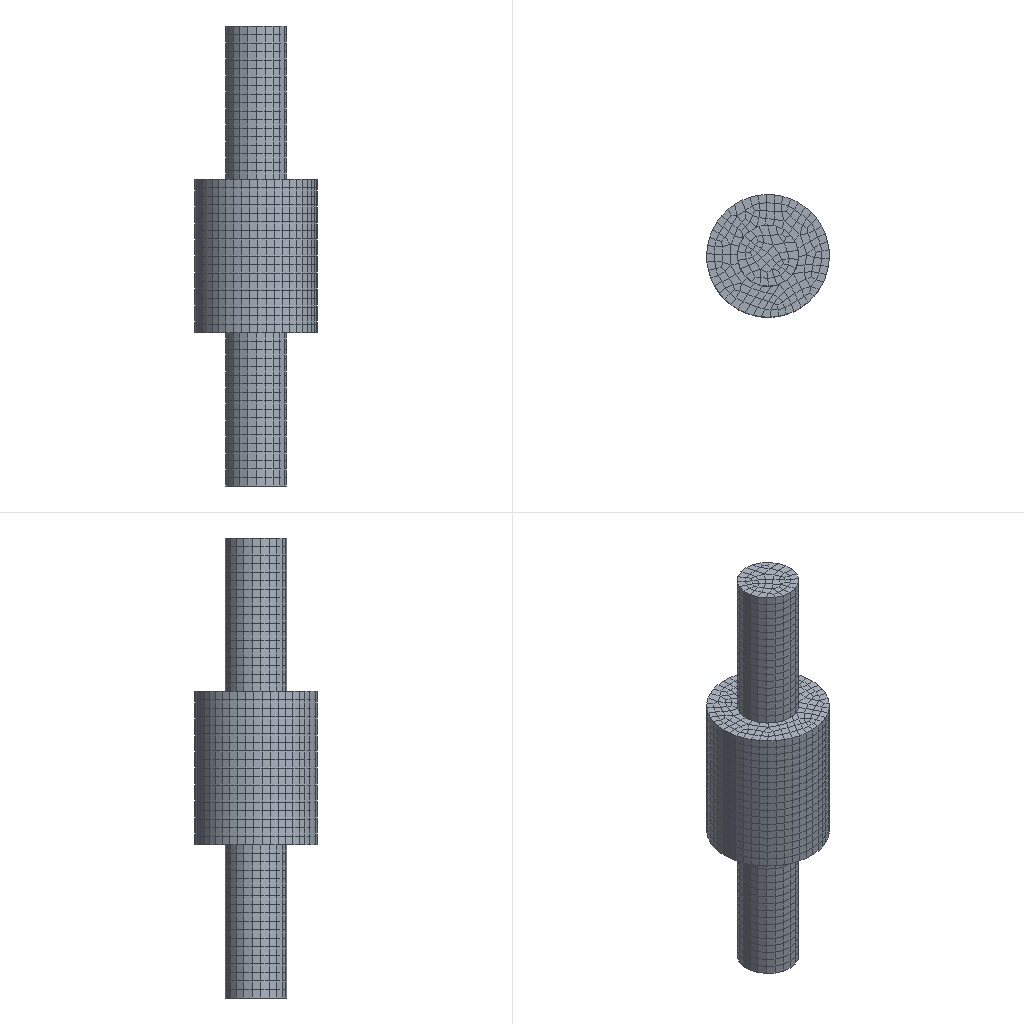Simulation study | abaqus
Set-up summary:
category,name,step,type,value,unit,region
solver,abaqus
solver,version,,,Abaqus/Standard 2020
units,not stated in the deck,,not stated
analysis,deck,,transient,transient
load_step,Step-1,Step-1,transient
load_step,requested,,,1
mesh,nodes,,,7238
mesh,elements,,,5724
element_type,C3D8R,,solid,5724
load,load commands in deck,,count,2
bc,support commands in deck,,count,6
material,MATERIAL-1,,in results
check,setup vs results,,match,"per instance, exact: element labels, types and connectivity; labels of the nodes the elements use; coordinates of those nodes at SINGLE_PRECISION in 2 of 2 instance(s)"
Abaqus input file, long lists of numbers shortened:
*Heading
** Job name: Job-1 Model name: Model-1
** Generated by: Abaqus/CAE 2020
*Preprint, echo=NO, model=NO, history=NO, contact=NO
**
** PARTS
**
*Part, name=Part-1
*Node
      1,   9.165,  -4.001,           0.
      2,   9.921,  -1.257,           0.
** (3683 more lines like these left out)
*Element, type=C3D8R
   1,  107,   89,   79,   91,   40,   22,   12,   24
   2,  106,   78,   88,   92,   39,   11,   21,   25
** (2968 more lines like these left out)
*Nset, nset=Set-1, generate
    1,  3685,     1
*Elset, elset=Set-1, generate
    1,  2970,     1
** Section: Section-1
*Solid Section, elset=Set-1, material=Material-1
,
*End Part
**
*Part, name=tong
*Node
      1,   8.194,  -5.732,           0.
      2,   9.477,  -3.192,           0.
** (3551 more lines like these left out)
*Element, type=C3D8R
   1,  301,  233,  191,  259,  114,   46,    4,   72
   2,  356,  308,  257,  337,  169,  121,   70,  150
** (2752 more lines like these left out)
*Nset, nset=Set-1, generate
    1,  3553,     1
*Elset, elset=Set-1, generate
    1,  2754,     1
** Section: Section-1
*Solid Section, elset=Set-1, material=Material-1
,
*End Part
**
**
** ASSEMBLY
**
*Assembly, name=Assembly
**
*Instance, name=Part-1-1, part=Part-1
*End Instance
**
*Instance, name=tong-1, part=tong
          0.,           0.,          50.
*End Instance
**
*Node
      1,           0.,           0.,          75.
*Nset, nset=Set-1, instance=Part-1-1, generate
    1,  3685,     1
*Elset, elset=Set-1, instance=Part-1-1, generate
    1,  2970,     1
*Nset, nset=Set-3
 1,
*Nset, nset=m_Set-2
 1,
*Elset, elset=_Surf-3_S4, internal, instance=Part-1-1
    1,    2,   16,   18,   19,   20,   21,   22,   23,   24,   50,   51,   52,   56,   57,   71
   73,   74,   75,   76,   77,   78,   79,  105,  106,  107,  111,  112,  126,  128,  129,  130
** (42 more lines like these left out)
*Elset, elset=_Surf-3_S3, internal, instance=Part-1-1
    8,   25,   28,   29,   63,   80,   83,   84,  118,  135,  138,  139,  173,  190,  193,  194
  228,  245,  248,  249,  283,  300,  303,  304,  338,  355,  358,  359,  393,  410,  413,  414
** (12 more lines like these left out)
*Elset, elset=_Surf-3_S6, internal, instance=Part-1-1
    9,   10,   17,   26,   36,   64,   65,   72,   81,   91,  119,  120,  127,  136,  146,  174
  175,  182,  191,  201,  229,  230,  237,  246,  256,  284,  285,  292,  301,  311,  339,  340
** (15 more lines like these left out)
*Surface, type=ELEMENT, name=Surf-3
_Surf-3_S4, S4
_Surf-3_S3, S3
_Surf-3_S6, S6
*Elset, elset=_m_Surf-1_S4, internal, instance=tong-1
    1,   25,   66,   70,   79,   85,   86,   99,  154,  178,  219,  223,  232,  238,  239,  252
  307,  331,  372,  376,  385,  391,  392,  405,  460,  484,  525,  529,  538,  544,  545,  558
** (7 more lines like these left out)
*Elset, elset=_m_Surf-1_S6, internal, instance=tong-1
    5,    6,    8,   24,   27,   41,   45,  158,  159,  161,  177,  180,  194,  198,  311,  312
  314,  330,  333,  347,  351,  464,  465,  467,  483,  486,  500,  504,  617,  618,  620,  636
** (6 more lines like these left out)
*Elset, elset=_m_Surf-1_S5, internal, instance=tong-1
   13,   35,  166,  188,  319,  341,  472,  494,  625,  647,  778,  800,  931,  953, 1084, 1106
 1237, 1259, 1390, 1412, 1543, 1565, 1696, 1718, 1849, 1871, 2002, 2024, 2155, 2177, 2308, 2330
** (1 more lines like these left out)
*Elset, elset=_m_Surf-1_S3, internal, instance=tong-1
   71,   81,   91,   95,   96,  224,  234,  244,  248,  249,  377,  387,  397,  401,  402,  530
  540,  550,  554,  555,  683,  693,  703,  707,  708,  836,  846,  856,  860,  861,  989,  999
** (4 more lines like these left out)
*Surface, type=ELEMENT, name=m_Surf-1
_m_Surf-1_S4, S4
_m_Surf-1_S6, S6
_m_Surf-1_S5, S5
_m_Surf-1_S3, S3
*Elset, elset=_s_Surf-1_S4, internal, instance=Part-1-1
    1,    2,   16,   18,   19,   20,   21,   22,   23,   24,   50,   51,   52,   56,   57,   71
   73,   74,   75,   76,   77,   78,   79,  105,  106,  107,  111,  112,  126,  128,  129,  130
** (42 more lines like these left out)
*Elset, elset=_s_Surf-1_S3, internal, instance=Part-1-1
    8,   25,   28,   29,   63,   80,   83,   84,  118,  135,  138,  139,  173,  190,  193,  194
  228,  245,  248,  249,  283,  300,  303,  304,  338,  355,  358,  359,  393,  410,  413,  414
** (12 more lines like these left out)
*Elset, elset=_s_Surf-1_S6, internal, instance=Part-1-1
    9,   10,   17,   26,   36,   64,   65,   72,   81,   91,  119,  120,  127,  136,  146,  174
  175,  182,  191,  201,  229,  230,  237,  246,  256,  284,  285,  292,  301,  311,  339,  340
** (15 more lines like these left out)
*Surface, type=ELEMENT, name=s_Surf-1
_s_Surf-1_S4, S4
_s_Surf-1_S3, S3
_s_Surf-1_S6, S6
*Elset, elset=_s_Surf-4_S1, internal, instance=Part-1-1, generate
 2916,  2970,     1
*Elset, elset=_s_Surf-4_S2, internal, instance=Part-1-1, generate
  1,  55,   1
*Surface, type=ELEMENT, name=s_Surf-4
_s_Surf-4_S1, S1
_s_Surf-4_S2, S2
** Constraint: Constraint-1
*Coupling, constraint name=Constraint-1, ref node=m_Set-2, surface=s_Surf-4
*Kinematic
*End Assembly
*Amplitude, name=Amp-1
             0.,              0.,             10.,              1.
**
** MATERIALS
**
*Material, name=Material-1
*Density
 7.8e-09,
*Elastic
210000., 0.3
**
** INTERACTION PROPERTIES
**
*Surface Interaction, name=IntProp-1
1.,
*Friction, slip tolerance=0.005
 0.1,
*Surface Behavior, pressure-overclosure=HARD
**
** INTERACTIONS
**
** Interaction: Int-1
*Contact Pair, interaction=IntProp-1, type=SURFACE TO SURFACE
s_Surf-1, m_Surf-1
** ----------------------------------------------------------------
**
** STEP: Step-1
**
*Step, name=Step-1, nlgeom=YES, inc=1000
*Dynamic
0.1,10.,0.0001
**
** BOUNDARY CONDITIONS
**
** Name: BC-1 Type: 位移/转角
*Boundary, amplitude=Amp-1
Set-3, 1, 1
Set-3, 2, 2
Set-3, 3, 3
Set-3, 4, 4
Set-3, 5, 5
Set-3, 6, 6, 6.28
**
** LOADS
**
** Name: Load-1   Type: Pressure
*Dsload
Surf-3, P, -0.01
**
** OUTPUT REQUESTS
**
*Restart, write, frequency=0
**
** FIELD OUTPUT: F-Output-1
**
*Output, field, frequency=1
*Node Output
A, AR, AT, CF, RF, U, UR, UT
V, VR, VT
*Element Output, directions=YES
E, LE, MISES, MISESMAX, PE, PEEQ, PEMAG, S
*Contact Output
CDISP, CSTRESS
**
** HISTORY OUTPUT: H-Output-1
**
*Output, history, variable=PRESELECT
*End Step
Results summary:
result,step,,partial,increments=100 time=10/10.0
result,analysis,,,transient
result,last_loadstep,,,1
result,primary field,,,U
result,reaction total,,FX,7.6e-05,model units
result,reaction total,,FY,-1e-05,model units
result,reaction total,,FZ,0.0,model units